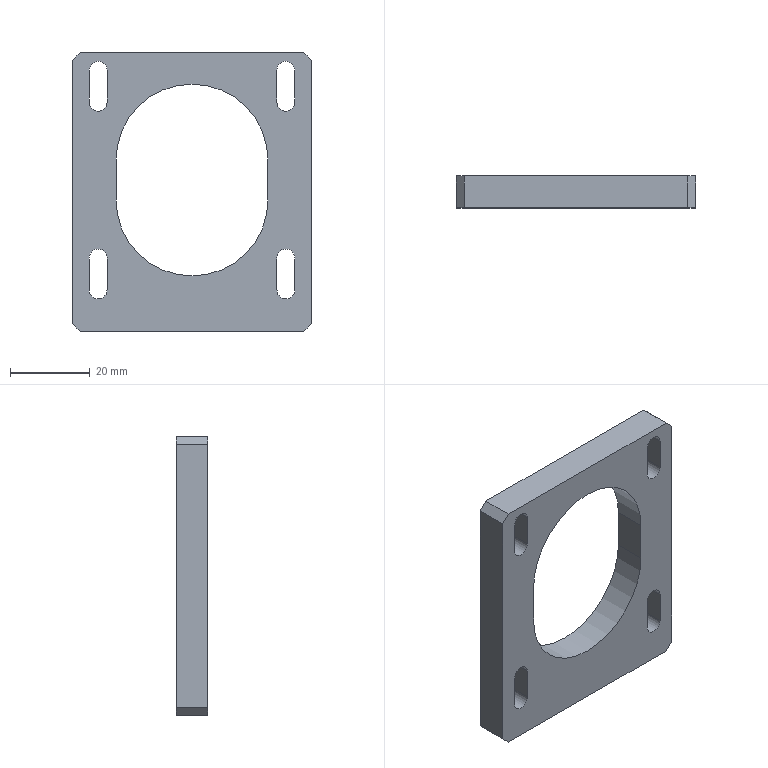Part | STEP file | PN_0035 | 1 solid | 43 faces | box 60 x 8 x 70 mm | volume 19436 mm3 | plane 20 | cylinder 19 | cone 4 | commonest cylinder face diameters 4.5 x12 3.3 x4 38.1 x3